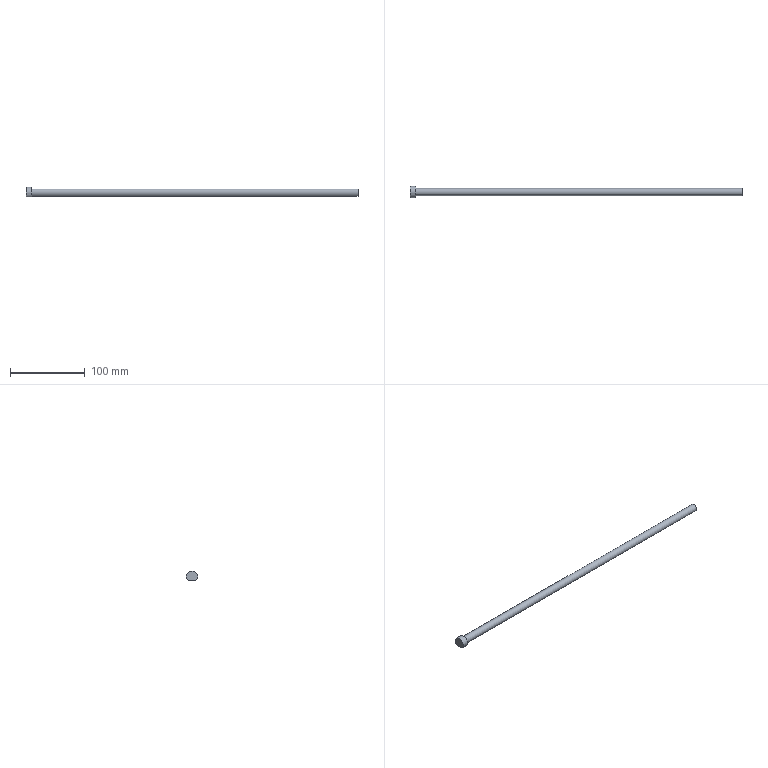Part | STEP file | solid 49 | 1 solid | 6 faces | box 445 x 15 x 13 mm | volume 35624 mm3 | plane 4 | cylinder 2 | commonest cylinder face diameters 10 x1 15 x1